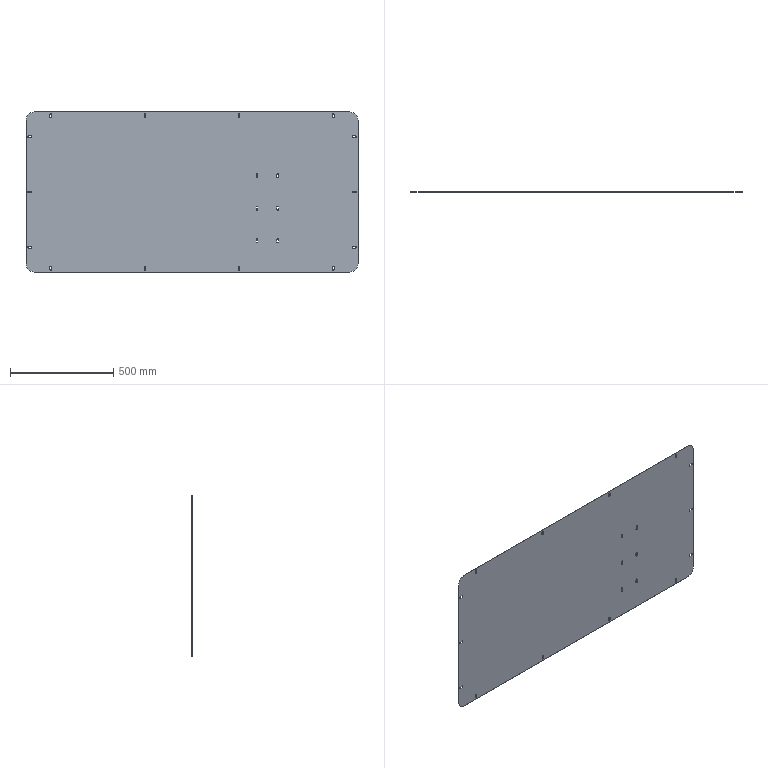Part | 1 solid | 104 faces | box 1606 x 1.2 x 774 mm | volume 1486376 mm3 | cylinder 58 | plane 46 | commonest cylinder face diameters 8.2 x54 80 x4